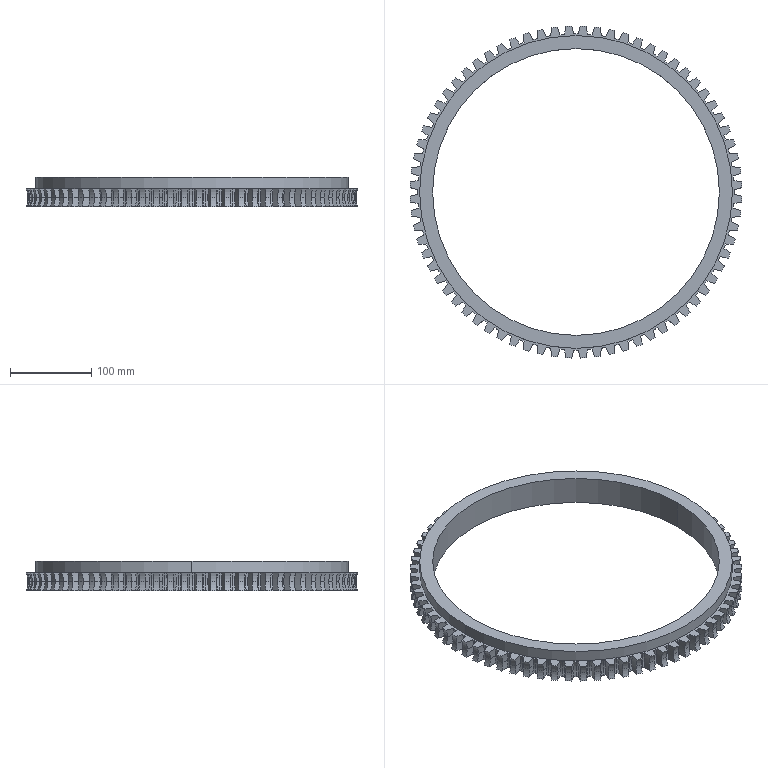Part | SolidWorks | features CirPattern 1, Revolution 1, SweepCut 1 | 1 solid | 509 faces | box 407.55 x 407.55 x 36 mm | volume 828010 mm3 | torus 288 | cone 214 | cylinder 4 | plane 3 | commonest cylinder face diameters 352 x2 384 x2